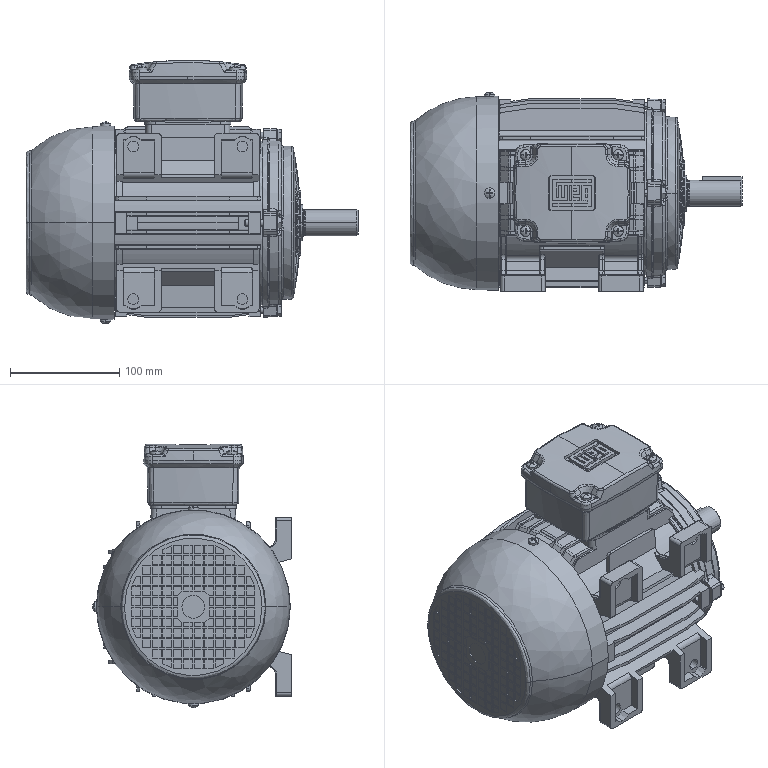Part | SolidWorks | features BaseBody 1 | 1 solid | 2034 faces | box 304.5 x 182.47 x 241.47 mm | volume 5604300 mm3 | plane 1131 | spline 464 | cylinder 273 | cone 162 | torus 4 | commonest cylinder face diameters 6 x76 2 x44 10 x44 4 x24 9.5 x14 286 x12